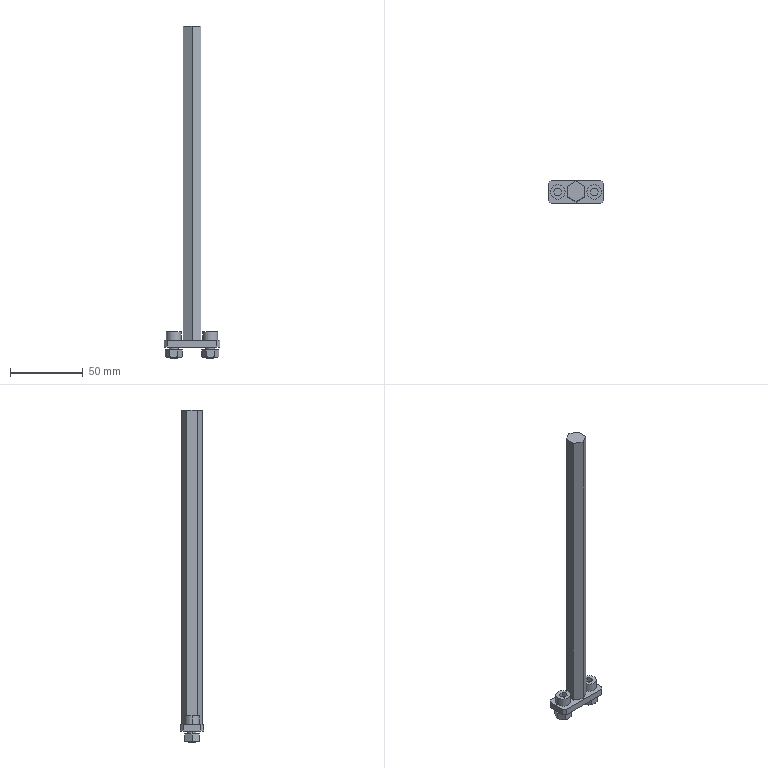Part | STEP file | ASND-0110-Q20_1 | 1 solid | 81 faces | box 38 x 16 x 227.5 mm | volume 31386 mm3 | plane 51 | cone 22 | cylinder 8 | commonest cylinder face diameters 6 x4 10 x4